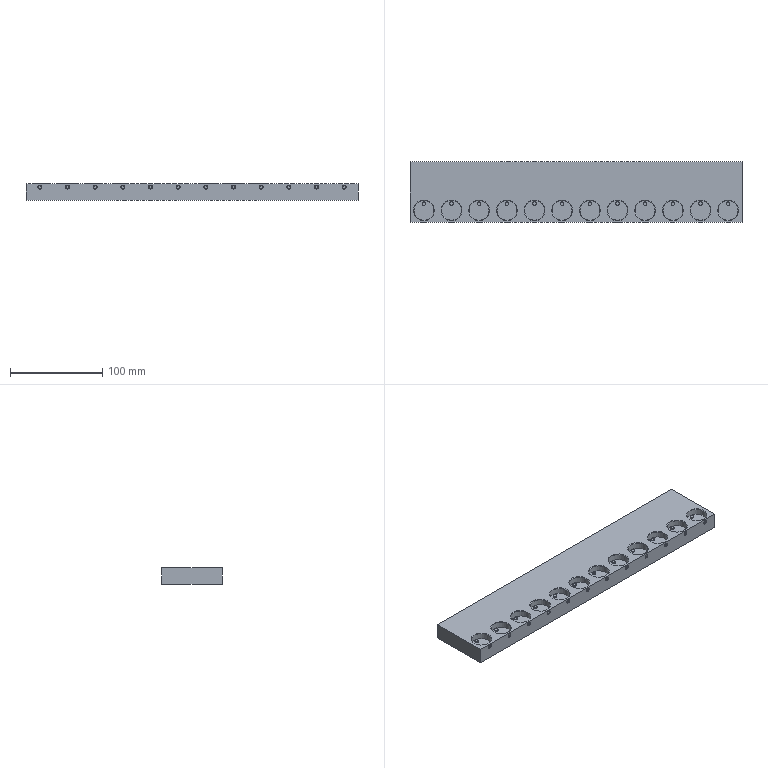NC program | NX | posted with a generic post | part box 360 x 66 x 17.6 mm
Lines 10620 to 11382 of 61781:
(3 , TOOL : D1-T3)
N21100 T03 M6
N21102 G54
N21104 G17 G0 G90 X-14.5 Y-2.81 B0. C0. S6500 M3
N21106 G43 Z100.15 H3
N21108 Z2.953
N21110 G94 G1 Z-0.047 F2500.
N21112 Y-2.797
N21114 G3 X-15. Y-2.297 R0.5
N21116 X-25.703 Y-13. R10.703
N21118 X-15. Y-2.297 R-10.703
N21120 G1 X-15.12 Y-2.3 Z-0.049
N21122 X-15.24 Y-2.304 Z-0.051
N21124 X-15.36 Y-2.31 Z-0.054
N21126 X-15.48 Y-2.316 Z-0.056
N21128 X-15.6 Y-2.325 Z-0.058
N21130 X-15.72 Y-2.334 Z-0.06
N21132 X-15.84 Y-2.345 Z-0.062
N21134 X-15.959 Y-2.357 Z-0.064
N21136 X-16.078 Y-2.371 Z-0.066
N21138 X-16.198 Y-2.386 Z-0.068
N21140 X-16.316 Y-2.402 Z-0.07
N21142 X-16.435 Y-2.419 Z-0.072
N21144 X-16.554 Y-2.438 Z-0.075
N21146 X-16.672 Y-2.458 Z-0.077
N21148 X-16.79 Y-2.48 Z-0.079
N21150 X-16.908 Y-2.503 Z-0.081
N21152 X-17.025 Y-2.527 Z-0.083
N21154 X-17.142 Y-2.552 Z-0.085
N21156 X-17.259 Y-2.579 Z-0.087
N21158 X-17.375 Y-2.607 Z-0.089
N21160 X-17.491 Y-2.637 Z-0.091
N21162 X-17.607 Y-2.667 Z-0.093
N21164 X-17.723 Y-2.699 Z-0.096
N21166 X-17.838 Y-2.733 Z-0.098
N21168 X-17.952 Y-2.767 Z-0.1
N21170 X-18.066 Y-2.803 Z-0.102
N21172 X-18.18 Y-2.84 Z-0.104
N21174 X-18.293 Y-2.878 Z-0.106
N21176 X-18.406 Y-2.918 Z-0.108
N21178 X-18.519 Y-2.959 Z-0.11
N21180 X-18.631 Y-3.001 Z-0.112
N21182 X-18.742 Y-3.044 Z-0.114
N21184 X-18.853 Y-3.089 Z-0.117
N21186 X-18.963 Y-3.135 Z-0.119
N21188 X-19.073 Y-3.182 Z-0.121
N21190 X-19.182 Y-3.23 Z-0.123
N21192 X-19.291 Y-3.28 Z-0.125
N21194 X-19.399 Y-3.331 Z-0.127
N21196 X-19.506 Y-3.383 Z-0.129
N21198 X-19.613 Y-3.436 Z-0.131
N21200 X-19.719 Y-3.49 Z-0.133
N21202 X-19.825 Y-3.545 Z-0.135
N21204 X-19.93 Y-3.602 Z-0.138
N21206 X-20.034 Y-3.66 Z-0.14
N21208 X-20.138 Y-3.719 Z-0.142
N21210 X-20.241 Y-3.779 Z-0.144
N21212 X-20.343 Y-3.84 Z-0.146
N21214 X-20.444 Y-3.903 Z-0.148
N21216 X-20.545 Y-3.966 Z-0.15
N21218 X-20.645 Y-4.031 Z-0.152
N21220 X-20.744 Y-4.097 Z-0.154
N21222 X-20.843 Y-4.164 Z-0.156
N21224 X-20.941 Y-4.231 Z-0.159
N21226 X-21.038 Y-4.3 Z-0.161
N21228 X-21.134 Y-4.371 Z-0.163
N21230 X-21.229 Y-4.442 Z-0.165
N21232 X-21.324 Y-4.514 Z-0.167
N21234 X-21.417 Y-4.587 Z-0.169
N21236 X-21.51 Y-4.661 Z-0.171
N21238 X-21.602 Y-4.737 Z-0.173
N21240 X-21.693 Y-4.813 Z-0.175
N21242 X-21.783 Y-4.89 Z-0.177
N21244 X-21.873 Y-4.969 Z-0.18
N21246 X-21.961 Y-5.048 Z-0.182
N21248 X-22.049 Y-5.128 Z-0.184
N21250 X-22.135 Y-5.21 Z-0.186
N21252 X-22.221 Y-5.292 Z-0.188
N21254 X-22.305 Y-5.375 Z-0.19
N21256 X-22.389 Y-5.459 Z-0.192
N21258 X-22.472 Y-5.544 Z-0.194
N21260 X-22.554 Y-5.63 Z-0.196
N21262 X-22.635 Y-5.717 Z-0.198
N21264 X-22.714 Y-5.804 Z-0.201
N21266 X-22.793 Y-5.893 Z-0.203
N21268 X-22.871 Y-5.982 Z-0.205
N21270 X-22.948 Y-6.072 Z-0.207
N21272 X-23.023 Y-6.163 Z-0.209
N21274 X-23.098 Y-6.255 Z-0.211
N21276 X-23.172 Y-6.348 Z-0.213
N21278 X-23.244 Y-6.442 Z-0.215
N21280 X-23.316 Y-6.536 Z-0.217
N21282 X-23.386 Y-6.631 Z-0.219
N21284 X-23.456 Y-6.727 Z-0.222
N21286 X-23.524 Y-6.824 Z-0.224
N21288 X-23.591 Y-6.921 Z-0.226
N21290 X-23.657 Y-7.019 Z-0.228
N21292 X-23.722 Y-7.118 Z-0.23
N21294 X-23.786 Y-7.217 Z-0.232
N21296 X-23.848 Y-7.318 Z-0.234
N21298 X-23.91 Y-7.418 Z-0.236
N21300 X-23.97 Y-7.52 Z-0.238
N21302 X-24.029 Y-7.622 Z-0.24
N21304 X-24.087 Y-7.725 Z-0.242
N21306 X-24.144 Y-7.829 Z-0.245
N21308 G3 X-15. Y-2.495 R-10.505
N21310 G1 X-15.12 Y-2.497 Z-0.247
N21312 X-15.24 Y-2.502 Z-0.249
N21314 X-15.36 Y-2.507 Z-0.251
N21316 X-15.48 Y-2.514 Z-0.253
N21318 X-15.6 Y-2.522 Z-0.255
N21320 X-15.72 Y-2.532 Z-0.257
N21322 X-15.84 Y-2.543 Z-0.259
N21324 X-15.959 Y-2.555 Z-0.261
N21326 X-16.078 Y-2.569 Z-0.263
N21328 X-16.197 Y-2.584 Z-0.266
N21330 X-16.316 Y-2.601 Z-0.268
N21332 X-16.435 Y-2.618 Z-0.27
N21334 X-16.553 Y-2.638 Z-0.272
N21336 X-16.672 Y-2.658 Z-0.274
N21338 X-16.789 Y-2.68 Z-0.276
N21340 X-16.907 Y-2.703 Z-0.278
N21342 X-17.024 Y-2.728 Z-0.28
N21344 X-17.141 Y-2.754 Z-0.282
N21346 X-17.258 Y-2.781 Z-0.284
N21348 X-17.374 Y-2.81 Z-0.287
N21350 X-17.49 Y-2.839 Z-0.289
N21352 X-17.606 Y-2.871 Z-0.291
N21354 X-17.721 Y-2.903 Z-0.293
N21356 X-17.836 Y-2.937 Z-0.295
N21358 X-17.95 Y-2.972 Z-0.297
N21360 X-18.064 Y-3.009 Z-0.299
N21362 X-18.178 Y-3.046 Z-0.301
N21364 X-18.291 Y-3.085 Z-0.303
N21366 X-18.404 Y-3.126 Z-0.305
N21368 X-18.516 Y-3.167 Z-0.308
N21370 X-18.627 Y-3.21 Z-0.31
N21372 X-18.738 Y-3.254 Z-0.312
N21374 X-18.849 Y-3.3 Z-0.314
N21376 X-18.959 Y-3.346 Z-0.316
N21378 X-19.068 Y-3.394 Z-0.318
N21380 X-19.177 Y-3.443 Z-0.32
N21382 X-19.285 Y-3.494 Z-0.322
N21384 X-19.393 Y-3.545 Z-0.324
N21386 X-19.5 Y-3.598 Z-0.326
N21388 X-19.606 Y-3.652 Z-0.329
N21390 X-19.712 Y-3.707 Z-0.331
N21392 X-19.817 Y-3.764 Z-0.333
N21394 X-19.922 Y-3.821 Z-0.335
N21396 X-20.025 Y-3.88 Z-0.337
N21398 X-20.128 Y-3.94 Z-0.339
N21400 X-20.231 Y-4.001 Z-0.341
N21402 X-20.332 Y-4.063 Z-0.343
N21404 X-20.433 Y-4.127 Z-0.345
N21406 X-20.533 Y-4.191 Z-0.347
N21408 X-20.633 Y-4.257 Z-0.35
N21410 X-20.731 Y-4.324 Z-0.352
N21412 X-20.829 Y-4.392 Z-0.354
N21414 X-20.926 Y-4.461 Z-0.356
N21416 X-21.022 Y-4.531 Z-0.358
N21418 X-21.117 Y-4.602 Z-0.36
N21420 X-21.212 Y-4.674 Z-0.362
N21422 X-21.305 Y-4.747 Z-0.364
N21424 X-21.398 Y-4.822 Z-0.366
N21426 X-21.49 Y-4.897 Z-0.368
N21428 X-21.581 Y-4.974 Z-0.371
N21430 X-21.671 Y-5.051 Z-0.373
N21432 X-21.76 Y-5.129 Z-0.375
N21434 X-21.849 Y-5.209 Z-0.377
N21436 X-21.936 Y-5.289 Z-0.379
N21438 X-22.022 Y-5.371 Z-0.381
N21440 X-22.108 Y-5.453 Z-0.383
N21442 X-22.192 Y-5.537 Z-0.385
N21444 X-22.276 Y-5.621 Z-0.387
N21446 X-22.358 Y-5.706 Z-0.389
N21448 X-22.44 Y-5.792 Z-0.392
N21450 X-22.52 Y-5.879 Z-0.394
N21452 X-22.6 Y-5.967 Z-0.396
N21454 X-22.678 Y-6.056 Z-0.398
N21456 X-22.755 Y-6.146 Z-0.4
N21458 X-22.832 Y-6.237 Z-0.402
N21460 X-22.907 Y-6.328 Z-0.404
N21462 X-22.981 Y-6.42 Z-0.406
N21464 X-23.054 Y-6.513 Z-0.408
N21466 X-23.126 Y-6.607 Z-0.41
N21468 X-23.197 Y-6.702 Z-0.413
N21470 X-23.267 Y-6.797 Z-0.415
N21472 X-23.336 Y-6.894 Z-0.417
N21474 X-23.404 Y-6.991 Z-0.419
N21476 X-23.47 Y-7.089 Z-0.421
N21478 X-23.536 Y-7.187 Z-0.423
N21480 X-23.6 Y-7.286 Z-0.425
N21482 X-23.663 Y-7.386 Z-0.427
N21484 X-23.725 Y-7.487 Z-0.429
N21486 X-23.786 Y-7.588 Z-0.431
N21488 X-23.845 Y-7.69 Z-0.433
N21490 X-23.904 Y-7.793 Z-0.436
N21492 X-23.961 Y-7.896 Z-0.438
N21494 X-24.017 Y-8. Z-0.44
N21496 X-24.072 Y-8.105 Z-0.442
N21498 G3 X-15. Y-2.692 R-10.308
N21500 G1 X-15.12 Y-2.695 Z-0.444
N21502 X-15.24 Y-2.699 Z-0.446
N21504 X-15.36 Y-2.704 Z-0.448
N21506 X-15.48 Y-2.711 Z-0.45
N21508 X-15.6 Y-2.72 Z-0.452
N21510 X-15.72 Y-2.73 Z-0.454
N21512 X-15.84 Y-2.741 Z-0.457
N21514 X-15.959 Y-2.753 Z-0.459
N21516 X-16.078 Y-2.767 Z-0.461
N21518 X-16.197 Y-2.783 Z-0.463
N21520 X-16.316 Y-2.8 Z-0.465
N21522 X-16.435 Y-2.818 Z-0.467
N21524 X-16.553 Y-2.837 Z-0.469
N21526 X-16.671 Y-2.858 Z-0.471
N21528 X-16.789 Y-2.88 Z-0.473
N21530 X-16.907 Y-2.904 Z-0.475
N21532 X-17.024 Y-2.929 Z-0.478
N21534 X-17.141 Y-2.955 Z-0.48
N21536 X-17.257 Y-2.983 Z-0.482
N21538 X-17.373 Y-3.012 Z-0.484
N21540 X-17.489 Y-3.042 Z-0.486
N21542 X-17.605 Y-3.074 Z-0.488
N21544 X-17.72 Y-3.107 Z-0.49
N21546 X-17.834 Y-3.142 Z-0.492
N21548 X-17.949 Y-3.177 Z-0.494
N21550 X-18.062 Y-3.214 Z-0.496
N21552 X-18.176 Y-3.253 Z-0.499
N21554 X-18.289 Y-3.292 Z-0.501
N21556 X-18.402 Y-3.331 Z-0.503
N21558 X-18.514 Y-3.371 Z-0.505
N21560 X-18.626 Y-3.413 Z-0.507
N21562 X-18.738 Y-3.456 Z-0.509
N21564 X-18.849 Y-3.5 Z-0.511
N21566 X-18.96 Y-3.546 Z-0.513
N21568 X-19.07 Y-3.593 Z-0.515
N21570 X-19.179 Y-3.641 Z-0.517
N21572 X-19.288 Y-3.69 Z-0.52
N21574 X-19.396 Y-3.741 Z-0.522
N21576 X-19.504 Y-3.793 Z-0.524
N21578 X-19.611 Y-3.846 Z-0.526
N21580 X-19.718 Y-3.9 Z-0.528
N21582 X-19.823 Y-3.956 Z-0.53
N21584 X-19.929 Y-4.013 Z-0.532
N21586 X-20.033 Y-4.071 Z-0.534
N21588 X-20.137 Y-4.13 Z-0.536
N21590 X-20.24 Y-4.191 Z-0.538
N21592 X-20.342 Y-4.252 Z-0.541
N21594 X-20.444 Y-4.315 Z-0.543
N21596 X-20.545 Y-4.379 Z-0.545
N21598 X-20.645 Y-4.445 Z-0.547
N21600 X-20.745 Y-4.511 Z-0.549
N21602 X-20.843 Y-4.579 Z-0.551
N21604 X-20.941 Y-4.647 Z-0.553
N21606 X-21.038 Y-4.717 Z-0.555
N21608 X-21.134 Y-4.788 Z-0.557
N21610 X-21.23 Y-4.86 Z-0.559
N21612 X-21.324 Y-4.934 Z-0.562
N21614 X-21.418 Y-5.008 Z-0.564
N21616 X-21.511 Y-5.083 Z-0.566
N21618 X-21.603 Y-5.16 Z-0.568
N21620 X-21.694 Y-5.237 Z-0.57
N21622 X-21.784 Y-5.316 Z-0.572
N21624 X-21.873 Y-5.396 Z-0.574
N21626 X-21.961 Y-5.476 Z-0.576
N21628 X-22.048 Y-5.558 Z-0.578
N21630 X-22.135 Y-5.641 Z-0.58
N21632 X-22.22 Y-5.724 Z-0.583
N21634 X-22.304 Y-5.809 Z-0.585
N21636 X-22.388 Y-5.895 Z-0.587
N21638 X-22.47 Y-5.982 Z-0.589
N21640 X-22.552 Y-6.069 Z-0.591
N21642 X-22.632 Y-6.158 Z-0.593
N21644 X-22.711 Y-6.247 Z-0.595
N21646 X-22.789 Y-6.338 Z-0.597
N21648 X-22.867 Y-6.429 Z-0.599
N21650 X-22.943 Y-6.521 Z-0.601
N21652 X-23.018 Y-6.614 Z-0.604
N21654 X-23.092 Y-6.708 Z-0.606
N21656 X-23.165 Y-6.803 Z-0.608
N21658 X-23.236 Y-6.899 Z-0.61
N21660 X-23.307 Y-6.995 Z-0.612
N21662 X-23.376 Y-7.092 Z-0.614
N21664 X-23.445 Y-7.191 Z-0.616
N21666 X-23.512 Y-7.289 Z-0.618
N21668 X-23.578 Y-7.389 Z-0.62
N21670 X-23.643 Y-7.49 Z-0.622
N21672 X-23.706 Y-7.591 Z-0.624
N21674 X-23.769 Y-7.693 Z-0.627
N21676 X-23.83 Y-7.795 Z-0.629
N21678 X-23.89 Y-7.899 Z-0.631
N21680 X-23.949 Y-8.003 Z-0.633
N21682 X-24.007 Y-8.108 Z-0.635
N21684 X-24.063 Y-8.213 Z-0.637
N21686 X-24.119 Y-8.319 Z-0.639
N21688 G3 X-15. Y-2.75 R-10.25
N21690 G1 X-15.12 Y-2.751 Z-0.641
N21692 X-15.24 Y-2.753 Z-0.643
N21694 X-15.361 Y-2.756 Z-0.645
N21696 X-15.481 Y-2.761 Z-0.648
N21698 X-15.601 Y-2.768 Z-0.65
N21700 X-15.721 Y-2.775 Z-0.652
N21702 X-15.841 Y-2.785 Z-0.654
N21704 X-15.961 Y-2.795 Z-0.656
N21706 X-16.08 Y-2.807 Z-0.658
N21708 X-16.2 Y-2.82 Z-0.66
N21710 X-16.319 Y-2.835 Z-0.662
N21712 X-16.438 Y-2.851 Z-0.664
N21714 X-16.557 Y-2.869 Z-0.666
N21716 X-16.676 Y-2.888 Z-0.669
N21718 X-16.794 Y-2.908 Z-0.671
N21720 X-16.913 Y-2.93 Z-0.673
N21722 X-17.031 Y-2.953 Z-0.675
N21724 X-17.148 Y-2.978 Z-0.677
N21726 X-17.266 Y-3.004 Z-0.679
N21728 X-17.383 Y-3.031 Z-0.681
N21730 X-17.5 Y-3.059 Z-0.683
N21732 X-17.616 Y-3.089 Z-0.685
N21734 X-17.732 Y-3.121 Z-0.687
N21736 X-17.848 Y-3.154 Z-0.69
N21738 X-17.963 Y-3.188 Z-0.692
N21740 X-18.078 Y-3.223 Z-0.694
N21742 X-18.193 Y-3.26 Z-0.696
N21744 X-18.307 Y-3.298 Z-0.698
N21746 X-18.42 Y-3.337 Z-0.7
N21748 X-18.533 Y-3.378 Z-0.702
N21750 X-18.646 Y-3.42 Z-0.704
N21752 X-18.758 Y-3.464 Z-0.706
N21754 X-18.87 Y-3.509 Z-0.708
N21756 X-18.981 Y-3.555 Z-0.711
N21758 X-19.091 Y-3.602 Z-0.713
N21760 X-19.201 Y-3.651 Z-0.715
N21762 X-19.311 Y-3.701 Z-0.717
N21764 X-19.42 Y-3.752 Z-0.719
N21766 X-19.528 Y-3.804 Z-0.721
N21768 X-19.635 Y-3.858 Z-0.723
N21770 X-19.742 Y-3.913 Z-0.725
N21772 X-19.848 Y-3.969 Z-0.727
N21774 X-19.954 Y-4.027 Z-0.729
N21776 X-20.059 Y-4.085 Z-0.732
N21778 X-20.163 Y-4.145 Z-0.734
N21780 X-20.267 Y-4.207 Z-0.736
N21782 X-20.37 Y-4.269 Z-0.738
N21784 X-20.472 Y-4.333 Z-0.74
N21786 X-20.573 Y-4.397 Z-0.742
N21788 X-20.673 Y-4.463 Z-0.744
N21790 X-20.773 Y-4.53 Z-0.746
N21792 X-20.872 Y-4.599 Z-0.748
N21794 X-20.97 Y-4.668 Z-0.75
N21796 X-21.068 Y-4.739 Z-0.753
N21798 X-21.164 Y-4.811 Z-0.755
N21800 X-21.26 Y-4.883 Z-0.757
N21802 X-21.355 Y-4.957 Z-0.759
N21804 X-21.448 Y-5.033 Z-0.761
N21806 X-21.541 Y-5.109 Z-0.763
N21808 X-21.634 Y-5.186 Z-0.765
N21810 X-21.725 Y-5.264 Z-0.767
N21812 X-21.815 Y-5.344 Z-0.769
N21814 X-21.904 Y-5.424 Z-0.771
N21816 X-21.993 Y-5.506 Z-0.774
N21818 X-22.08 Y-5.588 Z-0.776
N21820 X-22.167 Y-5.672 Z-0.778
N21822 X-22.252 Y-5.757 Z-0.78
N21824 X-22.337 Y-5.842 Z-0.782
N21826 X-22.42 Y-5.929 Z-0.784
N21828 X-22.503 Y-6.016 Z-0.786
N21830 X-22.584 Y-6.105 Z-0.788
N21832 X-22.664 Y-6.194 Z-0.79
N21834 X-22.744 Y-6.285 Z-0.792
N21836 X-22.822 Y-6.376 Z-0.795
N21838 X-22.899 Y-6.468 Z-0.797
N21840 X-22.975 Y-6.561 Z-0.799
N21842 X-23.05 Y-6.655 Z-0.801
N21844 X-23.124 Y-6.75 Z-0.803
N21846 X-23.197 Y-6.846 Z-0.805
N21848 X-23.268 Y-6.942 Z-0.807
N21850 X-23.339 Y-7.04 Z-0.809
N21852 X-23.408 Y-7.138 Z-0.811
N21854 X-23.476 Y-7.237 Z-0.813
N21856 X-23.543 Y-7.337 Z-0.815
N21858 X-23.609 Y-7.437 Z-0.818
N21860 X-23.674 Y-7.539 Z-0.82
N21862 X-23.737 Y-7.641 Z-0.822
N21864 X-23.8 Y-7.744 Z-0.824
N21866 X-23.861 Y-7.847 Z-0.826
N21868 X-23.921 Y-7.952 Z-0.828
N21870 X-23.979 Y-8.057 Z-0.83
N21872 X-24.037 Y-8.162 Z-0.832
N21874 X-24.093 Y-8.269 Z-0.834
N21876 X-24.148 Y-8.376 Z-0.836
N21878 G3 X-15. Y-2.75 R-10.25
N21880 G1 X-15.12 Y-2.751 Z-0.839
N21882 X-15.24 Y-2.753 Z-0.841
N21884 X-15.361 Y-2.756 Z-0.843
N21886 X-15.481 Y-2.761 Z-0.845
N21888 X-15.601 Y-2.768 Z-0.847
N21890 X-15.721 Y-2.775 Z-0.849
N21892 X-15.841 Y-2.785 Z-0.851
N21894 X-15.961 Y-2.795 Z-0.853
N21896 X-16.08 Y-2.807 Z-0.855
N21898 X-16.2 Y-2.82 Z-0.857
N21900 X-16.319 Y-2.835 Z-0.86
N21902 X-16.438 Y-2.851 Z-0.862
N21904 X-16.557 Y-2.869 Z-0.864
N21906 X-16.676 Y-2.888 Z-0.866
N21908 X-16.794 Y-2.908 Z-0.868
N21910 X-16.913 Y-2.93 Z-0.87
N21912 X-17.031 Y-2.953 Z-0.872
N21914 X-17.148 Y-2.978 Z-0.874
N21916 X-17.266 Y-3.004 Z-0.876
N21918 X-17.383 Y-3.031 Z-0.878
N21920 X-17.5 Y-3.059 Z-0.881
N21922 X-17.616 Y-3.089 Z-0.883
N21924 X-17.732 Y-3.121 Z-0.885
N21926 X-17.848 Y-3.154 Z-0.887
N21928 X-17.963 Y-3.188 Z-0.889
N21930 X-18.078 Y-3.223 Z-0.891
N21932 X-18.193 Y-3.26 Z-0.893
N21934 X-18.307 Y-3.298 Z-0.895
N21936 X-18.42 Y-3.337 Z-0.897
N21938 X-18.533 Y-3.378 Z-0.899
N21940 X-18.646 Y-3.42 Z-0.902
N21942 X-18.758 Y-3.464 Z-0.904
N21944 X-18.87 Y-3.509 Z-0.906
N21946 X-18.981 Y-3.555 Z-0.908
N21948 X-19.091 Y-3.602 Z-0.91
N21950 X-19.201 Y-3.651 Z-0.912
N21952 X-19.311 Y-3.701 Z-0.914
N21954 X-19.42 Y-3.752 Z-0.916
N21956 X-19.528 Y-3.804 Z-0.918
N21958 X-19.635 Y-3.858 Z-0.92
N21960 X-19.742 Y-3.913 Z-0.923
N21962 X-19.848 Y-3.969 Z-0.925
N21964 X-19.954 Y-4.027 Z-0.927
N21966 X-20.059 Y-4.085 Z-0.929
N21968 X-20.163 Y-4.145 Z-0.931
N21970 X-20.267 Y-4.207 Z-0.933
N21972 X-20.37 Y-4.269 Z-0.935
N21974 X-20.472 Y-4.333 Z-0.937
N21976 X-20.573 Y-4.397 Z-0.939
N21978 X-20.673 Y-4.463 Z-0.941
N21980 X-20.773 Y-4.53 Z-0.944
N21982 X-20.872 Y-4.599 Z-0.946
N21984 X-20.97 Y-4.668 Z-0.948
N21986 X-21.068 Y-4.739 Z-0.95
N21988 X-21.164 Y-4.811 Z-0.952
N21990 X-21.26 Y-4.883 Z-0.954
N21992 X-21.355 Y-4.957 Z-0.956
N21994 X-21.448 Y-5.033 Z-0.958
N21996 X-21.541 Y-5.109 Z-0.96
N21998 X-21.634 Y-5.186 Z-0.962
N22000 X-21.725 Y-5.264 Z-0.965
N22002 X-21.815 Y-5.344 Z-0.967
N22004 X-21.904 Y-5.424 Z-0.969
N22006 X-21.993 Y-5.506 Z-0.971
N22008 X-22.08 Y-5.588 Z-0.973
N22010 X-22.167 Y-5.672 Z-0.975
N22012 X-22.252 Y-5.757 Z-0.977
N22014 X-22.337 Y-5.842 Z-0.979
N22016 X-22.42 Y-5.929 Z-0.981
N22018 X-22.503 Y-6.016 Z-0.983
N22020 X-22.584 Y-6.105 Z-0.986
N22022 X-22.664 Y-6.194 Z-0.988
N22024 X-22.744 Y-6.285 Z-0.99
N22026 X-22.822 Y-6.376 Z-0.992
N22028 X-22.899 Y-6.468 Z-0.994
N22030 X-22.975 Y-6.561 Z-0.996
N22032 X-23.05 Y-6.655 Z-0.998
N22034 X-23.124 Y-6.75 Z-1.
N22036 X-23.197 Y-6.846 Z-1.002
N22038 X-23.268 Y-6.942 Z-1.004
N22040 X-23.339 Y-7.04 Z-1.006
N22042 X-23.408 Y-7.138 Z-1.009
N22044 X-23.476 Y-7.237 Z-1.011
N22046 X-23.543 Y-7.337 Z-1.013
N22048 X-23.609 Y-7.437 Z-1.015
N22050 X-23.674 Y-7.539 Z-1.017
N22052 X-23.737 Y-7.641 Z-1.019
N22054 X-23.8 Y-7.744 Z-1.021
N22056 X-23.861 Y-7.847 Z-1.023
N22058 X-23.921 Y-7.952 Z-1.025
N22060 X-23.979 Y-8.057 Z-1.027
N22062 X-24.037 Y-8.162 Z-1.03
N22064 X-24.093 Y-8.269 Z-1.032
N22066 X-24.148 Y-8.376 Z-1.034
N22068 G3 X-15. Y-2.75 R-10.25
N22070 G1 X-15.12 Y-2.751 Z-1.036
N22072 X-15.24 Y-2.753 Z-1.038
N22074 X-15.361 Y-2.756 Z-1.04
N22076 X-15.481 Y-2.761 Z-1.042
N22078 X-15.601 Y-2.768 Z-1.044
N22080 X-15.721 Y-2.775 Z-1.046
N22082 X-15.841 Y-2.785 Z-1.048
N22084 X-15.961 Y-2.795 Z-1.051
N22086 X-16.08 Y-2.807 Z-1.053
N22088 X-16.2 Y-2.82 Z-1.055
N22090 X-16.319 Y-2.835 Z-1.057
N22092 X-16.438 Y-2.851 Z-1.059
N22094 X-16.557 Y-2.869 Z-1.061
N22096 X-16.676 Y-2.888 Z-1.063
N22098 X-16.794 Y-2.908 Z-1.065
N22100 X-16.913 Y-2.93 Z-1.067
N22102 X-17.031 Y-2.953 Z-1.069
N22104 X-17.148 Y-2.978 Z-1.072
N22106 X-17.266 Y-3.004 Z-1.074
N22108 X-17.383 Y-3.031 Z-1.076
N22110 X-17.5 Y-3.059 Z-1.078
N22112 X-17.616 Y-3.089 Z-1.08
N22114 X-17.732 Y-3.121 Z-1.082
N22116 X-17.848 Y-3.154 Z-1.084
N22118 X-17.963 Y-3.188 Z-1.086
N22120 X-18.078 Y-3.223 Z-1.088
N22122 X-18.193 Y-3.26 Z-1.09
N22124 X-18.307 Y-3.298 Z-1.093
N22126 X-18.42 Y-3.337 Z-1.095
N22128 X-18.533 Y-3.378 Z-1.097
N22130 X-18.646 Y-3.42 Z-1.099
N22132 X-18.758 Y-3.464 Z-1.101
N22134 X-18.87 Y-3.509 Z-1.103
N22136 X-18.981 Y-3.555 Z-1.105
N22138 X-19.091 Y-3.602 Z-1.107
N22140 X-19.201 Y-3.651 Z-1.109
N22142 X-19.311 Y-3.701 Z-1.111
N22144 X-19.42 Y-3.752 Z-1.114
N22146 X-19.528 Y-3.804 Z-1.116
N22148 X-19.635 Y-3.858 Z-1.118
N22150 X-19.742 Y-3.913 Z-1.12
N22152 X-19.848 Y-3.969 Z-1.122
N22154 X-19.954 Y-4.027 Z-1.124
N22156 X-20.059 Y-4.085 Z-1.126
N22158 X-20.163 Y-4.145 Z-1.128
N22160 X-20.267 Y-4.207 Z-1.13
N22162 X-20.37 Y-4.269 Z-1.132
N22164 X-20.472 Y-4.333 Z-1.135
N22166 X-20.573 Y-4.397 Z-1.137
N22168 X-20.673 Y-4.463 Z-1.139
N22170 X-20.773 Y-4.53 Z-1.141
N22172 X-20.872 Y-4.599 Z-1.143
N22174 X-20.97 Y-4.668 Z-1.145
N22176 X-21.068 Y-4.739 Z-1.147
N22178 X-21.164 Y-4.811 Z-1.149
N22180 X-21.26 Y-4.883 Z-1.151
N22182 X-21.355 Y-4.957 Z-1.153
N22184 X-21.448 Y-5.033 Z-1.156
N22186 X-21.541 Y-5.109 Z-1.158
N22188 X-21.634 Y-5.186 Z-1.16
N22190 X-21.725 Y-5.264 Z-1.162
N22192 X-21.815 Y-5.344 Z-1.164
N22194 X-21.904 Y-5.424 Z-1.166
N22196 X-21.993 Y-5.506 Z-1.168
N22198 X-22.08 Y-5.588 Z-1.17
N22200 X-22.167 Y-5.672 Z-1.172
N22202 X-22.252 Y-5.757 Z-1.174
N22204 X-22.337 Y-5.842 Z-1.177
N22206 X-22.42 Y-5.929 Z-1.179
N22208 X-22.503 Y-6.016 Z-1.181
N22210 X-22.584 Y-6.105 Z-1.183
N22212 X-22.664 Y-6.194 Z-1.185
N22214 X-22.744 Y-6.285 Z-1.187
N22216 X-22.822 Y-6.376 Z-1.189
N22218 X-22.899 Y-6.468 Z-1.191
N22220 X-22.975 Y-6.561 Z-1.193
N22222 X-23.05 Y-6.655 Z-1.195
N22224 X-23.124 Y-6.75 Z-1.197
N22226 X-23.197 Y-6.846 Z-1.2
N22228 X-23.268 Y-6.942 Z-1.202
N22230 X-23.339 Y-7.04 Z-1.204
N22232 X-23.408 Y-7.138 Z-1.206
N22234 X-23.476 Y-7.237 Z-1.208
N22236 X-23.543 Y-7.337 Z-1.21
N22238 X-23.609 Y-7.437 Z-1.212
N22240 X-23.674 Y-7.539 Z-1.214
N22242 X-23.737 Y-7.641 Z-1.216
N22244 X-23.8 Y-7.744 Z-1.218
N22246 X-23.861 Y-7.847 Z-1.221
N22248 X-23.921 Y-7.952 Z-1.223
N22250 X-23.979 Y-8.057 Z-1.225
N22252 X-24.037 Y-8.162 Z-1.227
N22254 X-24.093 Y-8.269 Z-1.229
N22256 X-24.148 Y-8.376 Z-1.231
N22258 G3 X-15. Y-2.75 R-10.25
N22260 G1 X-15.12 Y-2.751 Z-1.233
N22262 X-15.24 Y-2.753 Z-1.235
N22264 X-15.361 Y-2.756 Z-1.237
N22266 X-15.481 Y-2.761 Z-1.239
N22268 X-15.601 Y-2.768 Z-1.242
N22270 X-15.721 Y-2.775 Z-1.244
N22272 X-15.841 Y-2.785 Z-1.246
N22274 X-15.961 Y-2.795 Z-1.248
N22276 X-16.08 Y-2.807 Z-1.25
N22278 X-16.2 Y-2.82 Z-1.252
N22280 X-16.319 Y-2.835 Z-1.254
N22282 X-16.438 Y-2.851 Z-1.256
N22284 X-16.557 Y-2.869 Z-1.258
N22286 X-16.676 Y-2.888 Z-1.26
N22288 X-16.794 Y-2.908 Z-1.263
N22290 X-16.913 Y-2.93 Z-1.265
N22292 X-17.031 Y-2.953 Z-1.267
N22294 X-17.148 Y-2.978 Z-1.269
N22296 X-17.266 Y-3.004 Z-1.271
N22298 X-17.383 Y-3.031 Z-1.273
N22300 X-17.5 Y-3.059 Z-1.275
N22302 X-17.616 Y-3.089 Z-1.277
N22304 X-17.732 Y-3.121 Z-1.279
N22306 X-17.848 Y-3.154 Z-1.281
N22308 X-17.963 Y-3.188 Z-1.284
N22310 X-18.078 Y-3.223 Z-1.286
N22312 X-18.193 Y-3.26 Z-1.288
N22314 X-18.307 Y-3.298 Z-1.29
N22316 X-18.42 Y-3.337 Z-1.292
N22318 X-18.533 Y-3.378 Z-1.294
N22320 X-18.646 Y-3.42 Z-1.296
N22322 X-18.758 Y-3.464 Z-1.298
N22324 X-18.87 Y-3.509 Z-1.3
N22326 X-18.981 Y-3.555 Z-1.302
N22328 X-19.091 Y-3.602 Z-1.305
N22330 X-19.201 Y-3.651 Z-1.307
N22332 X-19.311 Y-3.701 Z-1.309
N22334 X-19.42 Y-3.752 Z-1.311
N22336 X-19.528 Y-3.804 Z-1.313
N22338 X-19.635 Y-3.858 Z-1.315
N22340 X-19.742 Y-3.913 Z-1.317
N22342 X-19.848 Y-3.969 Z-1.319
N22344 X-19.954 Y-4.027 Z-1.321
N22346 X-20.059 Y-4.085 Z-1.323
N22348 X-20.163 Y-4.145 Z-1.326
N22350 X-20.267 Y-4.207 Z-1.328
N22352 X-20.37 Y-4.269 Z-1.33
N22354 X-20.472 Y-4.333 Z-1.332
N22356 X-20.573 Y-4.397 Z-1.334
N22358 X-20.673 Y-4.463 Z-1.336
N22360 X-20.773 Y-4.53 Z-1.338
N22362 X-20.872 Y-4.599 Z-1.34
N22364 X-20.97 Y-4.668 Z-1.342
N22366 X-21.068 Y-4.739 Z-1.344
N22368 X-21.164 Y-4.811 Z-1.347
N22370 X-21.26 Y-4.883 Z-1.349
N22372 X-21.355 Y-4.957 Z-1.351
N22374 X-21.448 Y-5.033 Z-1.353
N22376 X-21.541 Y-5.109 Z-1.355
N22378 X-21.634 Y-5.186 Z-1.357
N22380 X-21.725 Y-5.264 Z-1.359
N22382 X-21.815 Y-5.344 Z-1.361
N22384 X-21.904 Y-5.424 Z-1.363
N22386 X-21.993 Y-5.506 Z-1.365
N22388 X-22.08 Y-5.588 Z-1.368
N22390 X-22.167 Y-5.672 Z-1.37
N22392 X-22.252 Y-5.757 Z-1.372
N22394 X-22.337 Y-5.842 Z-1.374
N22396 X-22.42 Y-5.929 Z-1.376
N22398 X-22.503 Y-6.016 Z-1.378
N22400 X-22.584 Y-6.105 Z-1.38
N22402 X-22.664 Y-6.194 Z-1.382
N22404 X-22.744 Y-6.285 Z-1.384
N22406 X-22.822 Y-6.376 Z-1.386
N22408 X-22.899 Y-6.468 Z-1.389
N22410 X-22.975 Y-6.561 Z-1.391
N22412 X-23.05 Y-6.655 Z-1.393
N22414 X-23.124 Y-6.75 Z-1.395
N22416 X-23.197 Y-6.846 Z-1.397
N22418 X-23.268 Y-6.942 Z-1.399
N22420 X-23.339 Y-7.04 Z-1.401
N22422 X-23.408 Y-7.138 Z-1.403
N22424 X-23.476 Y-7.237 Z-1.405
N22426 X-23.543 Y-7.337 Z-1.407
N22428 X-23.609 Y-7.437 Z-1.409
N22430 X-23.674 Y-7.539 Z-1.412
N22432 X-23.737 Y-7.641 Z-1.414
N22434 X-23.8 Y-7.744 Z-1.416
N22436 X-23.861 Y-7.847 Z-1.418
N22438 X-23.921 Y-7.952 Z-1.42
N22440 X-23.979 Y-8.057 Z-1.422
N22442 X-24.037 Y-8.162 Z-1.424
N22444 X-24.093 Y-8.269 Z-1.426
N22446 X-24.148 Y-8.376 Z-1.428
N22448 G3 X-15. Y-2.75 R-10.25
N22450 G1 X-15.12 Y-2.751 Z-1.43
N22452 X-15.24 Y-2.753 Z-1.433
N22454 X-15.361 Y-2.756 Z-1.435
N22456 X-15.481 Y-2.761 Z-1.437
N22458 X-15.601 Y-2.768 Z-1.439
N22460 X-15.721 Y-2.775 Z-1.441
N22462 X-15.841 Y-2.785 Z-1.443
N22464 X-15.961 Y-2.795 Z-1.445
N22466 X-16.08 Y-2.807 Z-1.447
N22468 X-16.2 Y-2.82 Z-1.449
N22470 X-16.319 Y-2.835 Z-1.451
N22472 X-16.438 Y-2.851 Z-1.454
N22474 X-16.557 Y-2.869 Z-1.456
N22476 X-16.676 Y-2.888 Z-1.458
N22478 X-16.794 Y-2.908 Z-1.46
N22480 X-16.913 Y-2.93 Z-1.462
N22482 X-17.031 Y-2.953 Z-1.464
N22484 X-17.148 Y-2.978 Z-1.466
N22486 X-17.266 Y-3.004 Z-1.468
N22488 X-17.383 Y-3.031 Z-1.47
N22490 X-17.5 Y-3.059 Z-1.472
N22492 X-17.616 Y-3.089 Z-1.475
N22494 X-17.732 Y-3.121 Z-1.477
N22496 X-17.848 Y-3.154 Z-1.479
N22498 X-17.963 Y-3.188 Z-1.481
N22500 X-18.078 Y-3.223 Z-1.483
N22502 X-18.193 Y-3.26 Z-1.485
N22504 X-18.307 Y-3.298 Z-1.487
N22506 X-18.42 Y-3.337 Z-1.489
N22508 X-18.533 Y-3.378 Z-1.491
N22510 X-18.646 Y-3.42 Z-1.493
N22512 X-18.758 Y-3.464 Z-1.496
N22514 X-18.87 Y-3.509 Z-1.498
N22516 X-18.981 Y-3.555 Z-1.5
N22518 X-19.091 Y-3.602 Z-1.502
N22520 X-19.201 Y-3.651 Z-1.504
N22522 X-19.311 Y-3.701 Z-1.506
N22524 X-19.42 Y-3.752 Z-1.508
N22526 X-19.528 Y-3.804 Z-1.51
N22528 X-19.635 Y-3.858 Z-1.512
N22530 X-19.742 Y-3.913 Z-1.514
N22532 X-19.848 Y-3.969 Z-1.517
N22534 X-19.954 Y-4.027 Z-1.519
N22536 X-20.059 Y-4.085 Z-1.521
N22538 X-20.163 Y-4.145 Z-1.523
N22540 X-20.267 Y-4.207 Z-1.525
N22542 X-20.37 Y-4.269 Z-1.527
N22544 X-20.472 Y-4.333 Z-1.529
N22546 X-20.573 Y-4.397 Z-1.531
N22548 X-20.673 Y-4.463 Z-1.533
N22550 X-20.773 Y-4.53 Z-1.535
N22552 X-20.872 Y-4.599 Z-1.538
N22554 X-20.97 Y-4.668 Z-1.54
N22556 X-21.068 Y-4.739 Z-1.542
N22558 X-21.164 Y-4.811 Z-1.544
N22560 X-21.26 Y-4.883 Z-1.546
N22562 X-21.355 Y-4.957 Z-1.548
N22564 X-21.448 Y-5.033 Z-1.55
N22566 X-21.541 Y-5.109 Z-1.552
N22568 X-21.634 Y-5.186 Z-1.554
N22570 X-21.725 Y-5.264 Z-1.556
N22572 X-21.815 Y-5.344 Z-1.559
N22574 X-21.904 Y-5.424 Z-1.561
N22576 X-21.993 Y-5.506 Z-1.563
N22578 X-22.08 Y-5.588 Z-1.565
N22580 X-22.167 Y-5.672 Z-1.567
N22582 X-22.252 Y-5.757 Z-1.569
N22584 X-22.337 Y-5.842 Z-1.571
N22586 X-22.42 Y-5.929 Z-1.573
N22588 X-22.503 Y-6.016 Z-1.575
N22590 X-22.584 Y-6.105 Z-1.577
N22592 X-22.664 Y-6.194 Z-1.58
N22594 X-22.744 Y-6.285 Z-1.582
N22596 X-22.822 Y-6.376 Z-1.584
N22598 X-22.899 Y-6.468 Z-1.586
N22600 X-22.975 Y-6.561 Z-1.588
N22602 X-23.05 Y-6.655 Z-1.59
N22604 X-23.124 Y-6.75 Z-1.592
N22606 X-23.197 Y-6.846 Z-1.594
N22608 X-23.268 Y-6.942 Z-1.596
N22610 X-23.339 Y-7.04 Z-1.598
N22612 X-23.408 Y-7.138 Z-1.6
N22614 X-23.476 Y-7.237 Z-1.603
N22616 X-23.543 Y-7.337 Z-1.605
N22618 X-23.609 Y-7.437 Z-1.607